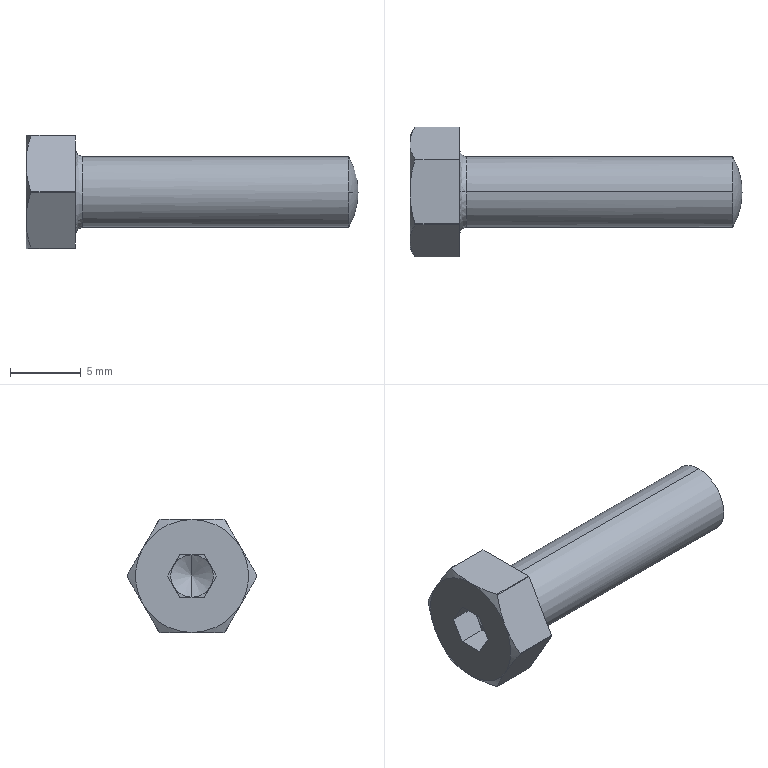Part | STEP file | 1_2 | 1 solid | 40 faces | box 23.5 x 9.2 x 8 mm | volume 562.948 mm3 | plane 20 | cylinder 8 | cone 8 | spline 4 | commonest cylinder face diameters 9.2 x6 5 x2